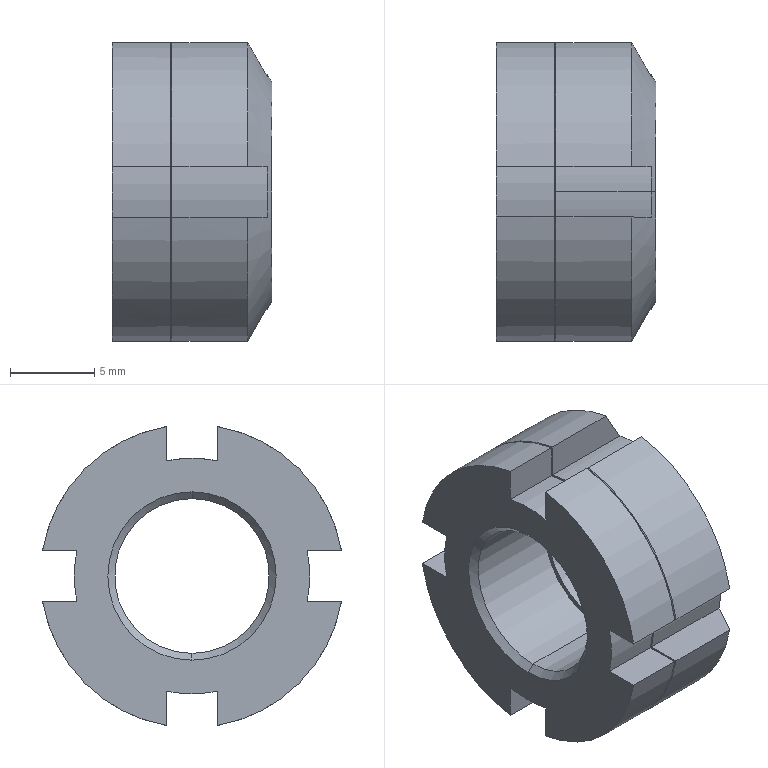Part | STEP file | 11-HLB1011_HLB10 | 1 solid | 79 faces | box 9.5 x 17.748 x 17.748 mm | volume 1479 mm3 | plane 36 | cylinder 27 | cone 16 | commonest cylinder face diameters 14 x10 18 x8 13.9 x5 9.188 x4